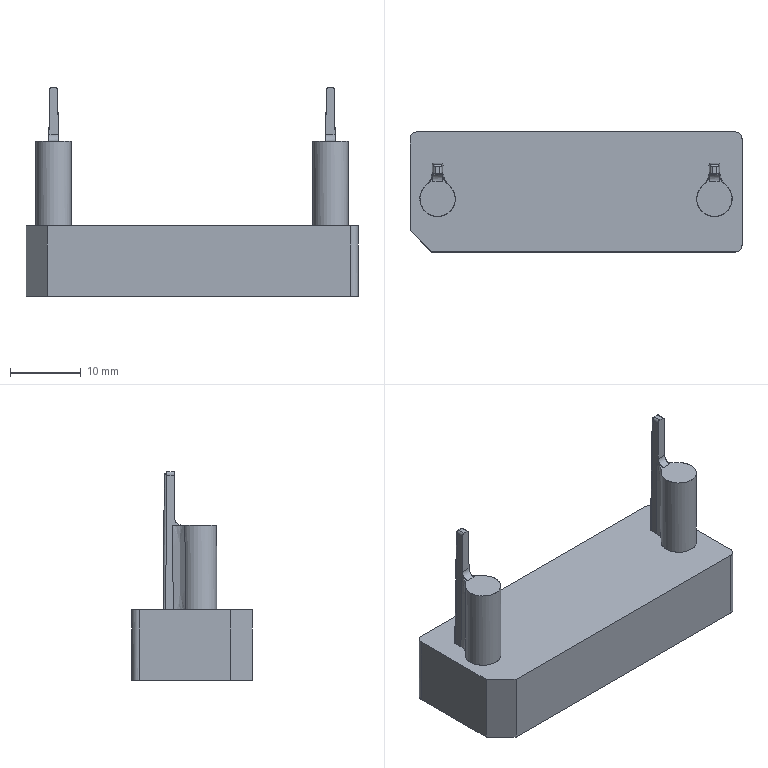NC program | PowerMill | posted with a generic post | part box 47 x 17 x 29.578 mm
Lines 1 to 1022 of 182382:
%
O0001
N104 ( POWERMILL CB  : 2026004.0)
N105 ( POST VER      : 2026.0.0.5161)
N106 ( OPTION FILE   : FANUC)
N107 ( OUTPUT WORKPLANE : WORLD)
N108 (  )
N109 ( TOOL LIST )
N110 (---------------------------------------)
N111 ( NO. | ID        | DIA.| TIP RAD|LENGTH)
N112 (---------------------------------------)
N113 (    1|D10C_1_1_1 |10.0 |  0.0   |85.04 )
N114 (    3|D10_1_1_1  |10.0 |  0.0   |84.72 )
N115 (   14|D4_2_1     | 4.0 |  0.0   | 74.6 )
N116 (   13|TEXT_D4_1_1| 4.0 |  0.3   |74.84 )
N117 (---------------------------------------)
N118 (  )
N119 ( NUMBER OF TOOLPATHS: 8.0 )
N120 ( ESTIMATED PROGRAM DURATION: 0 HOURS 16 MIN 0 SEC)
N121 (  )
N122 G00 G21 G80 G40 G17
N123 G90
N124 G54
N125 G53 Z0.0
N126 (---------------)
N127 ( START TOOLPATH : 粗公开粗01-扫面平行-D10C )
N128 (---------------)
N129 ( TOOL NO.    :1 )
N130 ( TOOL TYPE   : ENDMILL)
N131 ( TOOL ID     : D10C_1_1_1)
N132 ( TOOL DIA    : 10.0 LENGTH 85.04)
N133 T1
N134 M6
N135 S8000 M03
N136 G00 G90 X0.0 Y0.0
N137 G43 Z10.2 H1
N138
N139 G05 P10000 R4
N140 X31.15 Y11.15
N141 Z1.199
N142 G01 Z-0.001 F6000.0
N143 X26.15 F10000.0
N144 X-26.15
N145 Y5.575
N146 X26.15
N147 Y0.0
N148 X-26.15
N149 Y-5.575
N150 X26.15
N151 Y-11.15
N152 X-26.15
N153 X-31.15
N154 Z-0.202
N155 X-26.15
N156 X26.15
N157 Y-5.575
N158 X-26.15
N159 Y0.0
N160 X26.15
N161 Y5.575
N162 X-26.15
N163 Y11.15
N164 X26.15
N165 X31.15
N166 G00 Z10.2
N167 G05 P0
N168 (---------------)
N169 ( END TOOLPATH : 粗公开粗01-扫面平行-D10C )
N170 (---------------)
N171 ( START TOOLPATH : 粗公开粗01-外形偏置-D10C )
N172 (---------------)
N173 G00 X0.0005 Y0.2935 Z9.7981
N174 G05 P10000 R4
N175 X-24.6874 Y17.012
N176 Z0.5507
N177 G01 Z-0.6493 F6000.0
N178 Y16.4845 F10000.0
N179 G03 X-19.9399 Y11.737 I4.7475 J0.0
N180 G01 X18.908
N181 X18.9494 Y9.043
N182 X19.7229 Y9.0549
N183 X20.4963 Y9.0198
N184 X21.2697 Y8.8776
N185 X22.0432 Y8.6133
N186 X22.4536 Y8.4145
N187 X22.8166 Y8.202
N188 X23.5982 Y7.6411
N189 X24.3634 Y7.0411
N190 X24.5443 Y6.8676
N191 X25.1369 Y6.1812
N192 X25.6714 Y5.3208
N193 X26.003 Y4.5473
N194 X26.218 Y3.7739
N195 X26.3283 Y3.0005
N196 X26.3322 Y2.2271
N197 X26.2471 Y1.4536
N198 X26.0672 Y0.6802
N199 X25.9103 Y0.2421
N200 X25.759 Y-0.0932
N201 X25.3249 Y-0.8666
N202 X25.1369 Y-1.1481
N203 X24.7226 Y-1.6401
N204 X24.3634 Y-2.0072
N205 X23.8742 Y-2.4135
N206 X23.59 Y-2.6095
N207 X22.8166 Y-3.0454
N208 X22.4912 Y-3.1869
N209 X22.0432 Y-3.3471
N210 X21.2697 Y-3.5344
N211 X20.4963 Y-3.6228
N212 X18.9494 Y-3.633
N213 X18.176 Y-3.5764
N214 X17.4026 Y-3.4201
N215 X16.7004 Y-3.1869
N216 X15.8557 Y-2.767
N217 X15.325 Y-2.4135
N218 X15.0823 Y-2.218
N219 X14.4678 Y-1.6401
N220 X14.3089 Y-1.4625
N221 X13.8638 Y-0.8666
N222 X13.4282 Y-0.0932
N223 X13.1293 Y0.6802
N224 X12.9471 Y1.4536
N225 X12.8546 Y2.2271
N226 X12.8701 Y3.0005
N227 X12.9771 Y3.7739
N228 X13.192 Y4.5473
N229 X13.5236 Y5.3208
N230 X13.9948 Y6.0942
N231 X14.3089 Y6.497
N232 X14.6507 Y6.8676
N233 X15.0823 Y7.2597
N234 X15.5969 Y7.6411
N235 X16.6292 Y8.3522
N236 X17.4026 Y8.7141
N237 X18.176 Y8.935
N238 X18.9494 Y9.043
N239 X18.908 Y11.737
N240 X28.746
N241 G02 X29.746 Y10.737 I0.0 J-1.0
N242 G01 Y-10.15
N243 G02 X28.746 Y-11.15 I-1.0 J0.0
N244 G01 X-0.0027
N245 Y-5.6182
N246 Y-1.1182
N247 Y-5.6182
N248 X-7.0569
N249 G02 X-8.7104 Y-3.2115 I0.0 J1.7714
N250 G01 X-8.1242 Y-1.6856
N251 G03 X-7.4013 Y1.3615 I-10.9474 J4.2063
N252 G01 X-7.119 Y4.2041
N253 G02 X-5.1298 Y6.0064 I1.9902 J-0.1976
N254 G01 X5.1183 Y6.0119
N255 G02 X7.1098 Y4.2071 I0.001 J-2.0
N256 G01 X7.4236 Y1.0647
N257 X7.5607 Y0.2439
N258 G03 X8.1233 Y-1.7065 I11.3519 J2.2183
N259 G01 X8.7056 Y-3.2134
N260 G02 X7.0567 Y-5.6182 I-1.6489 J-0.6371
N261 G01 X-0.0027
N262 Y-11.15
N263 X-28.745
N264 G02 X-29.745 Y-10.15 I0.0 J1.0
N265 G01 Y10.737
N266 G02 X-28.745 Y11.737 I1.0 J0.0
N267 G01 X-19.9399
N268 X-19.8186 Y9.0505
N269 X-19.7219 Y9.0549
N270 X-18.9484 Y9.0429
N271 X-18.175 Y8.9348
N272 X-17.4016 Y8.7138
N273 X-16.7414 Y8.4145
N274 X-15.8547 Y7.8262
N275 X-15.0813 Y7.2588
N276 X-14.6507 Y6.8676
N277 X-14.3079 Y6.4958
N278 X-13.9948 Y6.0942
N279 X-13.5345 Y5.3419
N280 X-13.192 Y4.5473
N281 X-12.977 Y3.7739
N282 X-12.8674 Y3.0005
N283 X-12.8543 Y2.2271
N284 X-12.9497 Y1.4536
N285 X-13.1337 Y0.6802
N286 X-13.5345 Y-0.3046
N287 X-13.8666 Y-0.8666
N288 X-14.3079 Y-1.4625
N289 X-14.4666 Y-1.6401
N290 X-15.0813 Y-2.2174
N291 X-15.3214 Y-2.4135
N292 X-15.8547 Y-2.7669
N293 X-16.7017 Y-3.1869
N294 X-17.4016 Y-3.42
N295 X-18.175 Y-3.5763
N296 X-18.9484 Y-3.633
N297 X-20.4953 Y-3.6228
N298 X-21.2687 Y-3.5345
N299 X-22.0422 Y-3.3472
N300 X-22.4955 Y-3.1869
N301 X-22.8156 Y-3.0453
N302 X-23.589 Y-2.6098
N303 X-23.8728 Y-2.4135
N304 X-24.3624 Y-2.0073
N305 X-24.7288 Y-1.6401
N306 X-25.1359 Y-1.149
N307 X-25.3337 Y-0.8666
N308 X-25.7668 Y-0.0932
N309 X-25.9093 Y0.2355
N310 X-26.0617 Y0.6802
N311 X-26.2546 Y1.4536
N312 X-26.3402 Y2.2271
N313 X-26.3248 Y3.0005
N314 X-26.218 Y3.7739
N315 X-26.003 Y4.5473
N316 X-25.6714 Y5.3208
N317 X-25.2002 Y6.0942
N318 X-24.5443 Y6.8676
N319 X-24.3624 Y7.042
N320 X-23.589 Y7.6472
N321 X-22.8156 Y8.2027
N322 X-22.4536 Y8.4145
N323 X-22.0422 Y8.6137
N324 X-21.2687 Y8.8778
N325 X-20.4953 Y9.02
N326 X-19.8186 Y9.0505
N327 X-19.9399 Y11.737
N328 G00 Z3.2035
N329 G01 X-24.6874 Y17.012
N330 G00 Z0.1535
N331 G01 Z-1.0465 F6000.0
N332 Y16.4845 F10000.0
N333 G03 X-19.9399 Y11.737 I4.7475 J0.0
N334 G01 X18.9281
N335 X18.9494 Y10.0641
N336 X19.7229 Y10.0739
N337 X20.4963 Y10.0444
N338 X21.0732 Y9.9613
N339 X22.0432 Y9.6979
N340 X22.8166 Y9.3758
N341 X23.1638 Y9.1879
N342 X23.59 Y8.9154
N343 X24.2137 Y8.4145
N344 X24.9391 Y7.6411
N345 X25.1369 Y7.3832
N346 X25.475 Y6.8676
N347 X25.8606 Y6.0942
N348 X26.1204 Y5.3208
N349 X26.2798 Y4.5473
N350 X26.3468 Y3.7739
N351 X26.3394 Y2.2271
N352 X26.2544 Y1.4536
N353 X26.0706 Y0.6802
N354 X26.0303 Y0.5774
N355 X25.9102 Y0.2421
N356 X25.8245 Y0.0521
N357 X25.7676 Y-0.0932
N358 X25.3369 Y-0.8666
N359 X25.1369 Y-1.1552
N360 X24.7347 Y-1.6401
N361 X24.3634 Y-2.0127
N362 X23.8819 Y-2.4135
N363 X23.59 Y-2.6174
N364 X22.8166 Y-3.052
N365 X22.5079 Y-3.1869
N366 X22.0432 Y-3.3538
N367 X21.2697 Y-3.5408
N368 X20.4963 Y-3.6297
N369 X18.9494 Y-3.6366
N370 X18.176 Y-3.5819
N371 X17.4026 Y-3.4269
N372 X16.6882 Y-3.1869
N373 X15.8557 Y-2.7735
N374 X15.315 Y-2.4135
N375 X15.0823 Y-2.2308
N376 X14.4603 Y-1.6401
N377 X14.4099 Y-1.5753
N378 X14.3089 Y-1.4625
N379 X13.9998 Y-1.0486
N380 X13.8581 Y-0.8666
N381 X13.4245 Y-0.0932
N382 X13.1253 Y0.6802
N383 X12.9407 Y1.4536
N384 X12.8522 Y2.2271
N385 X12.8467 Y3.7739
N386 X12.9152 Y4.5473
N387 X13.0731 Y5.3208
N388 X13.3344 Y6.0942
N389 X13.72 Y6.8676
N390 X14.2559 Y7.6411
N391 X14.9795 Y8.4145
N392 X15.8557 Y9.0817
N393 X16.6292 Y9.4945
N394 X17.4026 Y9.7778
N395 X18.1219 Y9.9613
N396 X18.9494 Y10.0641
N397 X18.9281 Y11.737
N398 X28.746
N399 G02 X29.746 Y10.737 I0.0 J-1.0
N400 G01 Y-10.15
N401 G02 X28.746 Y-11.15 I-1.0 J0.0
N402 G01 X0.0022
N403 Y-5.6182
N404 Y-1.1182
N405 Y-5.6182
N406 X-7.0647 Y-5.6181
N407 G02 X-8.7297 Y-3.1796 I0.0 J1.7877
N408 G01 X-8.129 Y-1.6429
N409 G03 X-7.3852 Y1.1528 I-11.9924 J4.6875
N410 G01 X-6.9242 Y4.2566
N411 G02 X-4.9408 Y5.9628 I1.9783 J-0.2938
N412 G01 X4.9895 Y5.9375
N413 G02 X6.9641 Y4.2219 I-0.0051 J-2.0
N414 G01 X7.5124 Y0.4743
N415 G03 X8.1193 Y-1.7097 I11.3526 J1.9783
N416 G01 X8.7024 Y-3.2149
N417 G02 X7.056 Y-5.6182 I-1.6464 J-0.6377
N418 G01 X0.0022
N419 Y-11.15
N420 X-28.745
N421 G02 X-29.745 Y-10.15 I0.0 J1.0
N422 G01 Y10.737
N423 G02 X-28.745 Y11.737 I1.0 J0.0
N424 G01 X-20.0756
N425 X-20.0119 Y10.0629
N426 X-19.7219 Y10.0739
N427 X-18.9484 Y10.064
N428 X-18.175 Y9.9714
N429 X-17.4016 Y9.7802
N430 X-16.6282 Y9.4952
N431 X-15.8547 Y9.0811
N432 X-15.0813 Y8.5053
N433 X-14.3079 Y7.7043
N434 X-13.72 Y6.8676
N435 X-13.5345 Y6.5289
N436 X-13.3347 Y6.0942
N437 X-13.0746 Y5.3208
N438 X-12.9206 Y4.5473
N439 X-12.8465 Y3.7739
N440 X-12.8512 Y2.2271
N441 X-12.9385 Y1.4536
N442 X-13.1275 Y0.6802
N443 X-13.4271 Y-0.0932
N444 X-13.5058 Y-0.2339
N445 X-13.5345 Y-0.3046
N446 X-13.7316 Y-0.638
N447 X-13.8593 Y-0.8666
N448 X-14.0173 Y-1.07
N449 X-14.3079 Y-1.4624
N450 X-14.4168 Y-1.5843
N451 X-14.4601 Y-1.6401
N452 X-15.0813 Y-2.2299
N453 X-15.3142 Y-2.4135
N454 X-15.8547 Y-2.7732
N455 X-16.687 Y-3.1869
N456 X-17.4016 Y-3.4266
N457 X-18.175 Y-3.5817
N458 X-18.9484 Y-3.6366
N459 X-20.4953 Y-3.6298
N460 X-21.2687 Y-3.541
N461 X-22.0422 Y-3.3542
N462 X-22.2259 Y-3.2822
N463 X-22.4955 Y-3.1869
N464 X-22.6964 Y-3.098
N465 X-22.8156 Y-3.0513
N466 X-23.589 Y-2.6181
N467 X-23.8805 Y-2.4135
N468 X-24.3624 Y-2.0133
N469 X-24.7351 Y-1.6401
N470 X-25.1359 Y-1.1557
N471 X-25.3382 Y-0.8666
N472 X-25.7705 Y-0.0932
N473 X-25.8015 Y-0.013
N474 X-25.9092 Y0.2355
N475 X-26.0012 Y0.5039
N476 X-26.0693 Y0.6802
N477 X-26.2579 Y1.4536
N478 X-26.3427 Y2.2271
N479 X-26.3485 Y3.7739
N480 X-26.2799 Y4.5473
N481 X-26.1219 Y5.3208
N482 X-25.9093 Y5.9728
N483 X-25.475 Y6.8676
N484 X-25.1359 Y7.3846
N485 X-24.939 Y7.6411
N486 X-24.3624 Y8.2743
N487 X-23.589 Y8.9161
N488 X-23.1638 Y9.1879
N489 X-22.8156 Y9.376
N490 X-22.0422 Y9.6981
N491 X-21.2687 Y9.9201
N492 X-20.4953 Y10.0445
N493 X-20.0119 Y10.0629
N494 X-20.0756 Y11.737
N495 X-19.9399
N496 G00 Z2.8062
N497 G01 X-24.6874 Y17.012
N498 G00 Z-0.2438
N499 G01 Z-1.4438 F6000.0
N500 Y16.4845 F10000.0
N501 G03 X-19.9399 Y11.737 I4.7475 J0.0
N502 G01 X18.929
N503 X18.9494 Y10.068
N504 X19.7229 Y10.0774
N505 X20.4963 Y10.0488
N506 X21.0938 Y9.9613
N507 X22.0432 Y9.7031
N508 X22.8166 Y9.3809
N509 X23.173 Y9.1879
N510 X23.59 Y8.9213
N511 X24.2227 Y8.4145
N512 X24.9412 Y7.6411
N513 X25.1369 Y7.3887
N514 X25.4805 Y6.8676
N515 X25.8655 Y6.0942
N516 X26.1263 Y5.3208
N517 X26.2798 Y4.5473
N518 X26.3491 Y3.7739
N519 X26.3458 Y2.2271
N520 X26.2609 Y1.4536
N521 X26.074 Y0.6802
N522 X25.9826 Y0.4443
N523 X25.9102 Y0.2422
N524 X25.8682 Y0.1491
N525 X25.7743 Y-0.0932
N526 X25.3426 Y-0.8666
N527 X25.1369 Y-1.1615
N528 X24.7413 Y-1.6401
N529 X24.3634 Y-2.0189
N530 X23.8885 Y-2.4135
N531 X23.59 Y-2.6232
N532 X22.8166 Y-3.0571
N533 X22.5197 Y-3.1869
N534 X22.0432 Y-3.3584
N535 X21.2697 Y-3.547
N536 X20.4963 Y-3.6333
N537 X18.9494 Y-3.6402
N538 X18.176 Y-3.5859
N539 X17.4026 Y-3.4313
N540 X16.676 Y-3.1869
N541 X15.8557 Y-2.7801
N542 X15.307 Y-2.4135
N543 X15.0823 Y-2.2371
N544 X14.4537 Y-1.6401
N545 X14.3594 Y-1.5188
N546 X14.309 Y-1.4624
N547 X14.1469 Y-1.2455
N548 X13.8524 Y-0.8666
N549 X13.4207 Y-0.0932
N550 X13.1211 Y0.6802
N551 X12.9344 Y1.4536
N552 X12.8492 Y2.2271
N553 X12.8456 Y3.7739
N554 X12.9151 Y4.5473
N555 X13.0687 Y5.3208
N556 X13.3295 Y6.0942
N557 X13.7145 Y6.8676
N558 X14.2538 Y7.6411
N559 X14.9723 Y8.4145
N560 X15.8557 Y9.0874
N561 X16.6292 Y9.4991
N562 X17.4026 Y9.7823
N563 X18.1009 Y9.9613
N564 X18.9494 Y10.068
N565 X18.929 Y11.737
N566 X28.746
N567 G02 X29.746 Y10.737 I0.0 J-1.0
N568 G01 Y-10.15
N569 G02 X28.746 Y-11.15 I-1.0 J0.0
N570 G01 X0.0394
N571 Y-5.6182
N572 Y-1.1182
N573 Y-5.6182
N574 X-7.0606
N575 G02 X-8.7 Y-3.219 I0.0 J1.7598
N576 G01 X-8.0979 Y-1.6752
N577 G03 X-7.0171 Y3.4353 I-14.953 J5.832
N578 G01 X-6.9906 Y4.0235
N579 G02 X-4.9982 Y5.9336 I1.9979 J-0.0899
N580 G01 X4.9374 Y5.9613
N581 G02 X6.9207 Y4.2588 I0.0055 J-2.0
N582 G01 X7.3889 Y1.1463
N583 G03 X8.1347 Y-1.6426 I12.767 J1.9204
N584 G01 X8.7366 Y-3.1789
N585 G02 X7.0724 Y-5.6181 I-1.6642 J-0.6519
N586 G01 X0.0394 Y-5.6182
N587 Y-11.15
N588 X-28.745
N589 G02 X-29.745 Y-10.15 I0.0 J1.0
N590 G01 Y10.737
N591 G02 X-28.745 Y11.737 I1.0 J0.0
N592 G01 X-20.0735
N593 X-20.0119 Y10.0668
N594 X-19.7219 Y10.0774
N595 X-18.9484 Y10.0679
N596 X-18.175 Y9.9755
N597 X-17.4016 Y9.7863
N598 X-16.6282 Y9.5
N599 X-15.8547 Y9.0867
N600 X-15.0813 Y8.5119
N601 X-14.3079 Y7.7062
N602 X-13.7145 Y6.8676
N603 X-13.659 Y6.7562
N604 X-13.5345 Y6.5288
N605 X-13.3978 Y6.2313
N606 X-13.3296 Y6.0942
N607 X-13.0687 Y5.3208
N608 X-12.9163 Y4.5473
N609 X-12.8454 Y3.7739
N610 X-12.8492 Y2.2271
N611 X-12.9341 Y1.4536
N612 X-13.1213 Y0.6802
N613 X-13.4208 Y-0.0932
N614 X-13.5233 Y-0.277
N615 X-13.5346 Y-0.3045
N616 X-13.6091 Y-0.4306
N617 X-13.8524 Y-0.8666
N618 X-14.156 Y-1.2573
N619 X-14.308 Y-1.4624
N620 X-14.3664 Y-1.5278
N621 X-14.4537 Y-1.6401
N622 X-15.0813 Y-2.2363
N623 X-15.3069 Y-2.4135
N624 X-15.8547 Y-2.7794
N625 X-16.6751 Y-3.1869
N626 X-17.4016 Y-3.431
N627 X-18.175 Y-3.5858
N628 X-18.9484 Y-3.6402
N629 X-20.4953 Y-3.6334
N630 X-21.2687 Y-3.5472
N631 X-22.0422 Y-3.3587
N632 X-22.3634 Y-3.2336
N633 X-22.4955 Y-3.1868
N634 X-22.5857 Y-3.1469
N635 X-22.8156 Y-3.0573
N636 X-23.589 Y-2.6239
N637 X-23.8881 Y-2.4135
N638 X-24.3624 Y-2.0198
N639 X-24.7414 Y-1.6401
N640 X-25.1359 Y-1.1625
N641 X-25.3426 Y-0.8666
N642 X-25.7743 Y-0.0932
N643 X-25.8387 Y0.073
N644 X-25.9092 Y0.2356
N645 X-25.967 Y0.4043
N646 X-26.0739 Y0.6802
N647 X-26.2611 Y1.4536
N648 X-26.3458 Y2.2271
N649 X-26.3501 Y3.7739
N650 X-26.2799 Y4.5473
N651 X-26.1263 Y5.3208
N652 X-25.9093 Y5.985
N653 X-25.4805 Y6.8676
N654 X-25.1359 Y7.3901
N655 X-24.9412 Y7.6411
N656 X-24.3624 Y8.2825
N657 X-23.589 Y8.922
N658 X-23.1731 Y9.1879
N659 X-22.8156 Y9.3814
N660 X-22.0422 Y9.7034
N661 X-21.2687 Y9.9244
N662 X-20.4953 Y10.0489
N663 X-20.0119 Y10.0668
N664 X-20.0735 Y11.737
N665 X-19.9399
N666 G00 Z2.4089
N667 G01 X-24.6874 Y17.012
N668 G00 Z-0.6411
N669 G01 Z-1.8411 F6000.0
N670 Y16.4845 F10000.0
N671 G03 X-19.9399 Y11.737 I4.7475 J0.0
N672 G01 X18.9295
N673 X18.9494 Y10.0717
N674 X19.7229 Y10.0809
N675 X20.4963 Y10.0528
N676 X21.1145 Y9.9613
N677 X22.0432 Y9.7078
N678 X22.8166 Y9.3861
N679 X23.1823 Y9.1879
N680 X23.59 Y8.9272
N681 X24.23 Y8.4145
N682 X24.9475 Y7.6411
N683 X25.1369 Y7.3968
N684 X25.486 Y6.8676
N685 X25.8704 Y6.0942
N686 X26.1307 Y5.3208
N687 X26.2827 Y4.5473
N688 X26.3527 Y3.7739
N689 X26.3494 Y2.2271
N690 X26.265 Y1.4536
N691 X26.0784 Y0.6802
N692 X25.9235 Y0.2796
N693 X25.9101 Y0.2422
N694 X25.9027 Y0.2256
N695 X25.7794 Y-0.0932
N696 X25.3484 Y-0.8666
N697 X25.1369 Y-1.169
N698 X24.7479 Y-1.6401
N699 X24.3634 Y-2.0255
N700 X23.8962 Y-2.4135
N701 X23.59 Y-2.629
N702 X22.8166 Y-3.0622
N703 X22.5314 Y-3.1869
N704 X22.0432 Y-3.363
N705 X21.2697 Y-3.5511
N706 X20.4963 Y-3.637
N707 X18.9494 Y-3.6437
N708 X18.176 Y-3.5898
N709 X17.4026 Y-3.4357
N710 X16.6292 Y-3.173
N711 X15.8557 Y-2.7857
N712 X15.6842 Y-2.6654
N713 X15.307 Y-2.4135
N714 X15.1582 Y-2.2966
N715 X15.0823 Y-2.2434
N716 X14.4471 Y-1.6401
N717 X14.31 Y-1.4635
N718 X14.309 Y-1.4624
N719 X14.3056 Y-1.4579
N720 X13.8466 Y-0.8666
N721 X13.4156 Y-0.0932
N722 X13.1166 Y0.6802
N723 X12.93 Y1.4536
N724 X12.8456 Y2.2271
N725 X12.8423 Y3.7739
N726 X12.9123 Y4.5473
N727 X13.0643 Y5.3208
N728 X13.3246 Y6.0942
N729 X13.709 Y6.8676
N730 X14.2475 Y7.6411
N731 X14.965 Y8.4145
N732 X15.8557 Y9.093
N733 X16.6292 Y9.5041
N734 X17.4026 Y9.7868
N735 X18.0799 Y9.9613
N736 X18.9494 Y10.0717
N737 X18.9295 Y11.737
N738 X28.746
N739 G02 X29.746 Y10.737 I0.0 J-1.0
N740 G01 Y-10.15
N741 G02 X28.746 Y-11.15 I-1.0 J0.0
N742 G01 X0.0004
N743 Y-5.6182
N744 Y-1.1182
N745 Y-5.6182
N746 X-7.05 Y-5.6181
N747 G02 X-8.7182 Y-3.1783 I0.0001 J1.7902
N748 G01 X-8.1189 Y-1.6391
N749 G03 X-7.3793 Y1.1471 I-12.0374 J4.6869
N750 G01 X-6.9167 Y4.2565
N751 G02 X-4.9335 Y5.9622 I1.9782 J-0.2942
N752 G01 X4.9861 Y5.9377
N753 G02 X6.9614 Y4.2183 I-0.0049 J-2.0
N754 G01 X7.4969 Y0.5039
N755 G03 X8.1113 Y-1.7175 I11.244 J1.9144
N756 G01 X8.6955 Y-3.2189
N757 G02 X7.0545 Y-5.6182 I-1.641 J-0.6385
N758 G01 X0.0004
N759 Y-11.15
N760 X-28.745
N761 G02 X-29.745 Y-10.15 I0.0 J1.0
N762 G01 Y10.737
N763 G02 X-28.745 Y11.737 I1.0 J0.0
N764 G01 X-20.0724
N765 X-20.0119 Y10.0704
N766 X-19.7219 Y10.0809
N767 X-18.9484 Y10.0716
N768 X-18.175 Y9.9797
N769 X-17.4016 Y9.7907
N770 X-16.6282 Y9.5045
N771 X-16.0126 Y9.1879
N772 X-15.921 Y9.1221
N773 X-15.8548 Y9.0867
N774 X-15.3527 Y8.7135
N775 X-15.0813 Y8.5184
N776 X-14.3079 Y7.7138
N777 X-13.709 Y6.8676
N778 X-13.5997 Y6.6477
N779 X-13.5346 Y6.5288
N780 X-13.4608 Y6.3684
N781 X-13.3246 Y6.0942
N782 X-13.0643 Y5.3208
N783 X-12.9123 Y4.5473
N784 X-12.8423 Y3.7739
N785 X-12.8456 Y2.2271
N786 X-12.93 Y1.4536
N787 X-13.1166 Y0.6802
N788 X-13.4156 Y-0.0932
N789 X-13.8466 Y-0.8666
N790 X-14.3079 Y-1.4822
N791 X-14.4061 Y-1.5788
N792 X-14.4537 Y-1.64
N793 X-14.8886 Y-2.0531
N794 X-15.0813 Y-2.2426
N795 X-15.2988 Y-2.4135
N796 X-15.8547 Y-2.7851
N797 X-16.6631 Y-3.1869
N798 X-17.4016 Y-3.4354
N799 X-18.175 Y-3.5897
N800 X-18.9484 Y-3.6437
N801 X-20.4953 Y-3.637
N802 X-21.2687 Y-3.5513
N803 X-22.0422 Y-3.3633
N804 X-22.8156 Y-3.0626
N805 X-23.589 Y-2.6296
N806 X-23.8962 Y-2.4135
N807 X-24.3624 Y-2.0264
N808 X-24.7479 Y-1.6401
N809 X-25.1359 Y-1.1703
N810 X-25.3484 Y-0.8666
N811 X-25.7794 Y-0.0932
N812 X-25.885 Y0.18
N813 X-25.9091 Y0.2356
N814 X-25.9295 Y0.2951
N815 X-26.0784 Y0.6802
N816 X-26.265 Y1.4536
N817 X-26.3494 Y2.2271
N818 X-26.3527 Y3.7739
N819 X-26.2827 Y4.5473
N820 X-26.1307 Y5.3208
N821 X-25.9093 Y5.9972
N822 X-25.486 Y6.8676
N823 X-25.1359 Y7.3981
N824 X-24.9475 Y7.6411
N825 X-24.3624 Y8.2893
N826 X-23.589 Y8.9279
N827 X-23.1823 Y9.1879
N828 X-22.8156 Y9.3866
N829 X-22.0422 Y9.7082
N830 X-21.2687 Y9.9286
N831 X-20.4953 Y10.0529
N832 X-20.0119 Y10.0704
N833 X-20.0724 Y11.737
N834 X-19.9399
N835 G00 Z2.0117
N836 G01 X-24.6874 Y17.012
N837 G00 Z-1.0383
N838 G01 Z-2.2383 F6000.0
N839 Y16.4845 F10000.0
N840 G03 X-19.9399 Y11.737 I4.7475 J0.0
N841 G01 X18.93
N842 X18.9494 Y10.0753
N843 X19.7229 Y10.0844
N844 X20.4963 Y10.0566
N845 X21.1351 Y9.9613
N846 X22.0432 Y9.7125
N847 X22.8166 Y9.3913
N848 X23.1915 Y9.1879
N849 X23.59 Y8.9331
N850 X24.2372 Y8.4145
N851 X24.9538 Y7.6411
N852 X25.1369 Y7.4048
N853 X25.4915 Y6.8676
N854 X25.8753 Y6.0942
N855 X26.1351 Y5.3208
N856 X26.2866 Y4.5473
N857 X26.3563 Y3.7739
N858 X26.353 Y2.2271
N859 X26.2691 Y1.4536
N860 X26.083 Y0.6802
N861 X25.7845 Y-0.0932
N862 X25.3541 Y-0.8666
N863 X25.1369 Y-1.177
N864 X24.7546 Y-1.6401
N865 X24.3634 Y-2.0322
N866 X23.9042 Y-2.4135
N867 X23.59 Y-2.6347
N868 X22.8166 Y-3.0672
N869 X22.5432 Y-3.1869
N870 X22.0432 Y-3.3675
N871 X21.2697 Y-3.5552
N872 X20.4963 Y-3.6406
N873 X18.9494 Y-3.6472
N874 X18.176 Y-3.5938
N875 X17.4026 Y-3.44
N876 X16.6516 Y-3.1869
N877 X15.8557 Y-2.7912
N878 X15.5052 Y-2.5458
N879 X15.307 Y-2.4134
N880 X15.2322 Y-2.3546
N881 X15.0823 Y-2.2497
N882 X14.4404 Y-1.6401
N883 X13.8409 Y-0.8666
N884 X13.4105 Y-0.0932
N885 X13.112 Y0.6802
N886 X12.9259 Y1.4536
N887 X12.842 Y2.2271
N888 X12.8387 Y3.7739
N889 X12.9084 Y4.5473
N890 X13.0599 Y5.3208
N891 X13.3197 Y6.0942
N892 X13.7035 Y6.8676
N893 X14.2412 Y7.6411
N894 X14.9578 Y8.4145
N895 X15.8557 Y9.0986
N896 X16.6292 Y9.5091
N897 X17.4026 Y9.7913
N898 X18.059 Y9.9613
N899 X18.9494 Y10.0753
N900 X18.93 Y11.737
N901 X28.746
N902 G02 X29.746 Y10.737 I0.0 J-1.0
N903 G01 Y-10.15
N904 G02 X28.746 Y-11.15 I-1.0 J0.0
N905 G01 X0.0004
N906 X0.0005 Y-5.6182
N907 Y-1.1182
N908 Y-5.6182
N909 X-7.0443 Y-5.6181
N910 G02 X-8.7131 Y-3.1781 I0.0001 J1.7907
N911 G01 X-8.1141 Y-1.6385
N912 G03 X-7.3752 Y1.1465 I-12.0433 J4.6857
N913 G01 X-6.9128 Y4.2564
N914 G02 X-4.9296 Y5.9622 I1.9782 J-0.2942
N915 G01 X4.9825 Y5.9376
N916 G02 X6.9577 Y4.218 I-0.005 J-2.0
N917 G01 X7.4923 Y0.507
N918 G03 X8.1063 Y-1.7168 I11.2471 J1.9086
N919 G01 X8.69 Y-3.2188
N920 G02 X7.0482 Y-5.6182 I-1.6418 J-0.638
N921 G01 X0.0005
N922 X0.0004 Y-11.15
N923 X-28.745
N924 G02 X-29.745 Y-10.15 I0.0 J1.0
N925 G01 Y10.737
N926 G02 X-28.745 Y11.737 I1.0 J0.0
N927 G01 X-20.0715
N928 X-20.0119 Y10.074
N929 X-19.7219 Y10.0844
N930 X-18.9484 Y10.0753
N931 X-18.175 Y9.9838
N932 X-17.4016 Y9.7951
N933 X-16.6282 Y9.5091
N934 X-16.0033 Y9.1879
N935 X-15.8847 Y9.1026
N936 X-15.8548 Y9.0866
N937 X-15.6262 Y8.9168
N938 X-15.0813 Y8.5249
N939 X-14.3079 Y7.7214
N940 X-13.7035 Y6.8676
N941 X-13.5423 Y6.5429
N942 X-13.5346 Y6.5288
N943 X-13.5255 Y6.5091
N944 X-13.3197 Y6.0942
N945 X-13.0599 Y5.3208
N946 X-12.9084 Y4.5473
N947 X-12.8387 Y3.7739
N948 X-12.842 Y2.2271
N949 X-12.9259 Y1.4536
N950 X-13.112 Y0.6802
N951 X-13.4105 Y-0.0932
N952 X-13.8409 Y-0.8666
N953 X-14.3079 Y-1.4898
N954 X-14.4306 Y-1.6102
N955 X-14.4538 Y-1.64
N956 X-14.6769 Y-1.852
N957 X-15.0813 Y-2.2489
N958 X-15.1561 Y-2.3013
N959 X-15.2989 Y-2.4135
N960 X-15.6801 Y-2.6683
N961 X-15.8547 Y-2.7906
N962 X-16.6512 Y-3.1869
N963 X-17.4016 Y-3.4398
N964 X-18.175 Y-3.5936
N965 X-18.9484 Y-3.6472
N966 X-20.4953 Y-3.6407
N967 X-21.2687 Y-3.5554
N968 X-22.0422 Y-3.3678
N969 X-22.8156 Y-3.0677
N970 X-23.589 Y-2.6354
N971 X-23.9042 Y-2.4135
N972 X-24.3624 Y-2.0331
N973 X-24.7546 Y-1.6401
N974 X-25.1359 Y-1.1784
N975 X-25.3541 Y-0.8666
N976 X-25.7845 Y-0.0932
N977 X-26.083 Y0.6802
N978 X-26.2691 Y1.4536
N979 X-26.353 Y2.2271
N980 X-26.3563 Y3.7739
N981 X-26.2866 Y4.5473
N982 X-26.1351 Y5.3208
N983 X-25.9093 Y6.0094
N984 X-25.4915 Y6.8676
N985 X-25.1359 Y7.4062
N986 X-24.9538 Y7.6411
N987 X-24.3624 Y8.2962
N988 X-23.589 Y8.9338
N989 X-23.1916 Y9.1879
N990 X-22.8156 Y9.3918
N991 X-22.0422 Y9.7128
N992 X-21.2687 Y9.9329
N993 X-20.4953 Y10.0567
N994 X-20.0119 Y10.074
N995 X-20.0715 Y11.737
N996 X-19.9399
N997 G00 Z1.6144
N998 G01 X-24.6874 Y17.012
N999 G00 Z-1.4356
N1000 G01 Z-2.6356 F6000.0
N1001 Y16.4845 F10000.0
N1002 G03 X-19.9399 Y11.737 I4.7475 J0.0
N1003 G01 X18.9304
N1004 X18.9494 Y10.079
N1005 X19.7229 Y10.0879
N1006 X20.4963 Y10.0604
N1007 X21.1558 Y9.9613
N1008 X22.0432 Y9.7171
N1009 X22.8166 Y9.3965
N1010 X23.2008 Y9.1879
N1011 X23.59 Y8.9389
N1012 X24.2445 Y8.4145
N1013 X24.9601 Y7.6411
N1014 X25.1369 Y7.4129
N1015 X25.497 Y6.8676
N1016 X25.8802 Y6.0942
N1017 X26.1395 Y5.3208
N1018 X26.2905 Y4.5473
N1019 X26.3598 Y3.7739
N1020 X26.3567 Y2.2271
N1021 X26.2731 Y1.4536
N1022 X26.0875 Y0.6802
N1023 X25.7896 Y-0.0932
N1024 X25.3599 Y-0.8666
N1025 X25.1369 Y-1.1851
N1026 X24.7612 Y-1.6401
N1027 X24.3634 Y-2.0388
N1028 X23.9123 Y-2.4135
N1029 X23.59 Y-2.6404
N1030 X22.8166 Y-3.0723
N1031 X22.555 Y-3.1869
N1032 X22.0432 Y-3.3721
N1033 X21.2697 Y-3.5593
N1034 X20.4963 Y-3.6442
N1035 X18.9494 Y-3.6507
N1036 X18.176 Y-3.5977
N1037 X17.4026 Y-3.4444
N1038 X16.6394 Y-3.1869
N1039 X15.8557 Y-2.7967
N1040 X15.3145 Y-2.4183
N1041 X15.307 Y-2.4134
N1042 X15.3044 Y-2.4113
N1043 X15.0823 Y-2.256
N1044 X14.4338 Y-1.6401
N1045 X13.8351 Y-0.8666
N1046 X13.4054 Y-0.0932
N1047 X13.1075 Y0.6802
N1048 X12.9219 Y1.4536
N1049 X12.8383 Y2.2271
N1050 X12.8352 Y3.7739
N1051 X12.9045 Y4.5473
N1052 X13.0555 Y5.3208
N1053 X13.3148 Y6.0942
N1054 X13.698 Y6.8676
N1055 X14.2349 Y7.6411
N1056 X14.9505 Y8.4145
N1057 X15.8557 Y9.1043
N1058 X16.6292 Y9.5141
N1059 X17.4026 Y9.7958
N1060 X18.0391 Y9.9613
N1061 X18.9494 Y10.079
N1062 X18.9304 Y11.737
N1063 X28.746
N1064 G02 X29.746 Y10.737 I0.0 J-1.0
N1065 G01 Y-10.15
N1066 G02 X28.746 Y-11.15 I-1.0 J0.0
N1067 G01 X0.0005
N1068 Y-5.6182
N1069 Y-1.1182
N1070 Y-5.6182
N1071 X-7.0386 Y-5.6181
N1072 G02 X-8.708 Y-3.1779 I0.0 J1.7911
N1073 G01 X-8.1093 Y-1.6379
N1074 G03 X-7.3712 Y1.146 I-12.049 J4.6844
N1075 G01 X-6.9089 Y4.2563
N1076 G02 X-4.9256 Y5.9622 I1.9783 J-0.2941
N1077 G01 X4.9788 Y5.9374
N1078 G02 X6.9541 Y4.2177 I-0.005 J-2.0
N1079 G01 X7.4877 Y0.5102
N1080 G03 X8.1012 Y-1.7161 I11.2501 J1.9026
N1081 G01 X8.6845 Y-3.2187
N1082 G02 X7.042 Y-5.6182 I-1.6425 J-0.6376
N1083 G01 X0.0005
N1084 Y-11.15
N1085 X-28.745
N1086 G02 X-29.745 Y-10.15 I0.0 J1.0
N1087 G01 Y10.737
N1088 G02 X-28.745 Y11.737 I1.0 J0.0
N1089 G01 X-20.0707
N1090 X-20.0119 Y10.0776
N1091 X-19.7219 Y10.0879
N1092 X-18.9484 Y10.0789
N1093 X-18.175 Y9.9879
N1094 X-17.4016 Y9.7995
N1095 X-16.6282 Y9.5138
N1096 X-15.994 Y9.1879
N1097 X-15.0813 Y8.5314
N1098 X-14.3079 Y7.729
N1099 X-13.698 Y6.8676
N1100 X-13.3148 Y6.0942
N1101 X-13.0555 Y5.3208
N1102 X-12.9045 Y4.5473
N1103 X-12.8352 Y3.7739
N1104 X-12.8383 Y2.2271
N1105 X-12.9219 Y1.4536
N1106 X-13.1075 Y0.6802
N1107 X-13.4054 Y-0.0932
N1108 X-13.8351 Y-0.8666
N1109 X-14.3079 Y-1.4973
N1110 X-15.0813 Y-2.2552
N1111 X-15.2291 Y-2.3586
N1112 X-15.2989 Y-2.4134
N1113 X-15.4938 Y-2.5437
N1114 X-15.8547 Y-2.7961
N1115 X-16.6392 Y-3.1869
N1116 X-17.4016 Y-3.4442
N1117 X-18.175 Y-3.5976
N1118 X-18.9484 Y-3.6507
N1119 X-20.4953 Y-3.6443